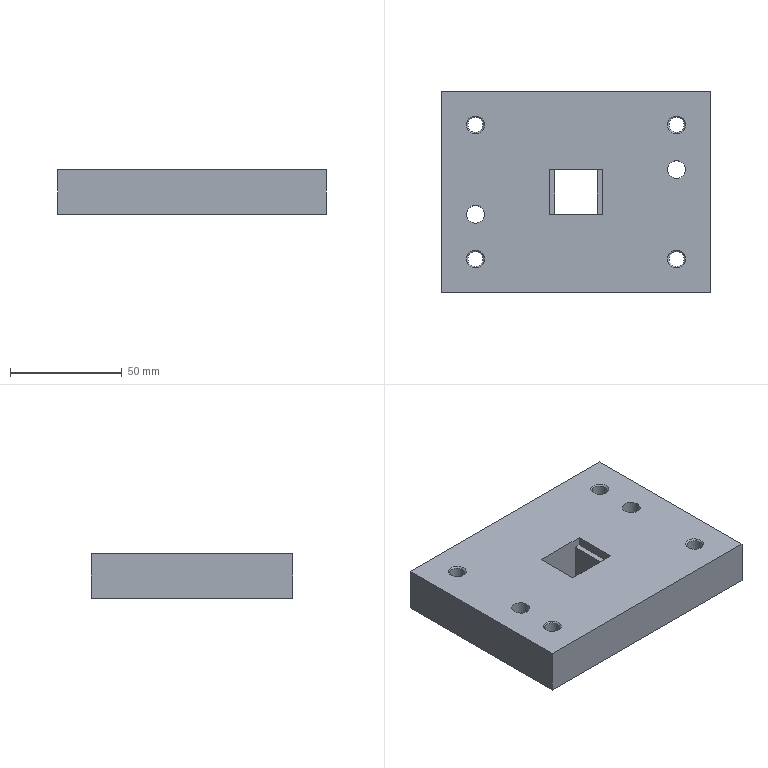Part | NX | features SIMPLE HOLE 4, SYMBOLIC_THREAD 4, EXTRUDE 2, DATUM_CSYS 1, HOLE PACKAGE 1 | 1 solid | 28 faces | box 120 x 90 x 20 mm | volume 203051 mm3 | plane 14 | cone 8 | cylinder 6 | commonest cylinder face diameters 6.8 x4 8 x2
STEP:
#1=CARTESIAN_POINT('',(-41.,-30.,0.));
#2=VERTEX_POINT('',#1);
#3=CARTESIAN_POINT('',(-45.,-30.,0.));
#4=DIRECTION('',(0.,0.,1.));
#5=DIRECTION('',(1.,0.,0.));
#6=AXIS2_PLACEMENT_3D('',#3,#4,#5);
#7=CIRCLE('',#6,4.);
#8=EDGE_CURVE('',#2,#2,#7,.F.);
#9=ORIENTED_EDGE('',*,*,#8,.T.);
#10=EDGE_LOOP('',(#9));
#11=FACE_BOUND('',#10,.T.);
#12=CARTESIAN_POINT('',(-41.,30.,0.));
#13=VERTEX_POINT('',#12);
#14=CARTESIAN_POINT('',(-45.,30.,0.));
#15=DIRECTION('',(0.,0.,1.));
#16=DIRECTION('',(1.,0.,0.));
#17=AXIS2_PLACEMENT_3D('',#14,#15,#16);
#18=CIRCLE('',#17,4.);
#19=EDGE_CURVE('',#13,#13,#18,.F.);
#20=ORIENTED_EDGE('',*,*,#19,.T.);
#21=EDGE_LOOP('',(#20));
#22=FACE_BOUND('',#21,.T.);
#23=CARTESIAN_POINT('',(49.,-30.,0.));
#24=VERTEX_POINT('',#23);
#25=CARTESIAN_POINT('',(45.,-30.,0.));
#26=DIRECTION('',(0.,0.,1.));
#27=DIRECTION('',(1.,0.,0.));
#28=AXIS2_PLACEMENT_3D('',#25,#26,#27);
#29=CIRCLE('',#28,4.);
#30=EDGE_CURVE('',#24,#24,#29,.F.);
#31=ORIENTED_EDGE('',*,*,#30,.T.);
#32=EDGE_LOOP('',(#31));
#33=FACE_BOUND('',#32,.T.);
#34=CARTESIAN_POINT('',(49.,30.,0.));
#35=VERTEX_POINT('',#34);
#36=CARTESIAN_POINT('',(45.,30.,0.));
#37=DIRECTION('',(0.,0.,1.));
#38=DIRECTION('',(1.,0.,0.));
#39=AXIS2_PLACEMENT_3D('',#36,#37,#38);
#40=CIRCLE('',#39,4.);
#41=EDGE_CURVE('',#35,#35,#40,.F.);
#42=ORIENTED_EDGE('',*,*,#41,.T.);
#43=EDGE_LOOP('',(#42));
#44=FACE_BOUND('',#43,.T.);
#45=CARTESIAN_POINT('',(60.,45.,0.));
#46=VERTEX_POINT('',#45);
#47=CARTESIAN_POINT('',(-60.,45.,0.));
#48=VERTEX_POINT('',#47);
#49=CARTESIAN_POINT('',(60.,45.,0.));
#50=DIRECTION('',(-1.,0.,0.));
#51=VECTOR('',#50,1000.);
#52=LINE('',#49,#51);
#53=EDGE_CURVE('',#46,#48,#52,.T.);
#54=ORIENTED_EDGE('',*,*,#53,.T.);
#55=CARTESIAN_POINT('',(-60.,-45.,0.));
#56=VERTEX_POINT('',#55);
#57=CARTESIAN_POINT('',(-60.,45.,0.));
#58=DIRECTION('',(0.,-1.,0.));
#59=VECTOR('',#58,1000.);
#60=LINE('',#57,#59);
#61=EDGE_CURVE('',#48,#56,#60,.T.);
#62=ORIENTED_EDGE('',*,*,#61,.T.);
#63=CARTESIAN_POINT('',(60.,-45.,0.));
#64=VERTEX_POINT('',#63);
#65=CARTESIAN_POINT('',(-60.,-45.,0.));
#66=DIRECTION('',(1.,0.,0.));
#67=VECTOR('',#66,1000.);
#68=LINE('',#65,#67);
#69=EDGE_CURVE('',#56,#64,#68,.T.);
#70=ORIENTED_EDGE('',*,*,#69,.T.);
#71=CARTESIAN_POINT('',(60.,-45.,0.));
#72=DIRECTION('',(0.,1.,0.));
#73=VECTOR('',#72,1000.);
#74=LINE('',#71,#73);
#75=EDGE_CURVE('',#64,#46,#74,.T.);
#76=ORIENTED_EDGE('',*,*,#75,.T.);
#77=EDGE_LOOP('',(#54,#62,#70,#76));
#78=FACE_BOUND('',#77,.T.);
#79=CARTESIAN_POINT('',(49.,10.,0.));
#80=VERTEX_POINT('',#79);
#81=CARTESIAN_POINT('',(45.,10.,0.));
#82=DIRECTION('',(0.,0.,1.));
#83=DIRECTION('',(1.,0.,0.));
#84=AXIS2_PLACEMENT_3D('',#81,#82,#83);
#85=CIRCLE('',#84,4.);
#86=EDGE_CURVE('',#80,#80,#85,.T.);
#87=ORIENTED_EDGE('',*,*,#86,.F.);
#88=EDGE_LOOP('',(#87));
#89=FACE_BOUND('',#88,.T.);
#90=CARTESIAN_POINT('',(-41.,-10.,0.));
#91=VERTEX_POINT('',#90);
#92=CARTESIAN_POINT('',(-45.,-10.,0.));
#93=DIRECTION('',(0.,0.,1.));
#94=DIRECTION('',(1.,0.,0.));
#95=AXIS2_PLACEMENT_3D('',#92,#93,#94);
#96=CIRCLE('',#95,4.);
#97=EDGE_CURVE('',#91,#91,#96,.T.);
#98=ORIENTED_EDGE('',*,*,#97,.F.);
#99=EDGE_LOOP('',(#98));
#100=FACE_BOUND('',#99,.T.);
#101=CARTESIAN_POINT('',(12.,-10.,0.));
#102=VERTEX_POINT('',#101);
#103=CARTESIAN_POINT('',(-12.,-10.,0.));
#104=VERTEX_POINT('',#103);
#105=CARTESIAN_POINT('',(9.5,-10.,0.));
#106=DIRECTION('',(-1.,0.,0.));
#107=VECTOR('',#106,1000.);
#108=LINE('',#105,#107);
#109=EDGE_CURVE('',#102,#104,#108,.T.);
#110=ORIENTED_EDGE('',*,*,#109,.T.);
#111=CARTESIAN_POINT('',(-12.,10.,0.));
#112=VERTEX_POINT('',#111);
#113=CARTESIAN_POINT('',(-12.,-10.,0.));
#114=DIRECTION('',(0.,1.,0.));
#115=VECTOR('',#114,1000.);
#116=LINE('',#113,#115);
#117=EDGE_CURVE('',#104,#112,#116,.T.);
#118=ORIENTED_EDGE('',*,*,#117,.T.);
#119=CARTESIAN_POINT('',(12.,10.,0.));
#120=VERTEX_POINT('',#119);
#121=CARTESIAN_POINT('',(-9.5,10.,0.));
#122=DIRECTION('',(1.,0.,0.));
#123=VECTOR('',#122,1000.);
#124=LINE('',#121,#123);
#125=EDGE_CURVE('',#112,#120,#124,.T.);
#126=ORIENTED_EDGE('',*,*,#125,.T.);
#127=CARTESIAN_POINT('',(12.,10.,0.));
#128=DIRECTION('',(0.,-1.,0.));
#129=VECTOR('',#128,1000.);
#130=LINE('',#127,#129);
#131=EDGE_CURVE('',#120,#102,#130,.T.);
#132=ORIENTED_EDGE('',*,*,#131,.T.);
#133=EDGE_LOOP('',(#110,#118,#126,#132));
#134=FACE_BOUND('',#133,.T.);
#135=CARTESIAN_POINT('',(45.,10.,0.));
#136=DIRECTION('',(0.,0.,1.));
#137=DIRECTION('',(1.,0.,0.));
#138=AXIS2_PLACEMENT_3D('',#135,#136,#137);
#139=PLANE('',#138);
#140=ADVANCED_FACE('',(#11,#22,#33,#44,#78,#89,#100,#134),#139,.T.);
#141=CARTESIAN_POINT('',(-9.5,-10.,-4.));
#142=VERTEX_POINT('',#141);
#143=CARTESIAN_POINT('',(-9.5,10.,-4.));
#144=VERTEX_POINT('',#143);
#145=CARTESIAN_POINT('',(-9.5,-10.,-4.));
#146=DIRECTION('',(0.,1.,0.));
#147=VECTOR('',#146,1000.);
#148=LINE('',#145,#147);
#149=EDGE_CURVE('',#142,#144,#148,.T.);
#150=ORIENTED_EDGE('',*,*,#149,.F.);
#151=CARTESIAN_POINT('',(-9.5,-10.,-20.));
#152=VERTEX_POINT('',#151);
#153=CARTESIAN_POINT('',(-9.5,-10.,-20.));
#154=DIRECTION('',(0.,0.,1.));
#155=VECTOR('',#154,1000.);
#156=LINE('',#153,#155);
#157=EDGE_CURVE('',#152,#142,#156,.T.);
#158=ORIENTED_EDGE('',*,*,#157,.F.);
#159=CARTESIAN_POINT('',(-9.5,10.,-20.));
#160=VERTEX_POINT('',#159);
#161=CARTESIAN_POINT('',(-9.5,-10.,-20.));
#162=DIRECTION('',(0.,1.,0.));
#163=VECTOR('',#162,1000.);
#164=LINE('',#161,#163);
#165=EDGE_CURVE('',#152,#160,#164,.T.);
#166=ORIENTED_EDGE('',*,*,#165,.T.);
#167=CARTESIAN_POINT('',(-9.5,10.,-20.));
#168=DIRECTION('',(0.,0.,1.));
#169=VECTOR('',#168,1000.);
#170=LINE('',#167,#169);
#171=EDGE_CURVE('',#160,#144,#170,.T.);
#172=ORIENTED_EDGE('',*,*,#171,.T.);
#173=EDGE_LOOP('',(#150,#158,#166,#172));
#174=FACE_BOUND('',#173,.T.);
#175=CARTESIAN_POINT('',(-9.5,-10.,-20.));
#176=DIRECTION('',(1.,0.,0.));
#177=DIRECTION('',(0.,0.,-1.));
#178=AXIS2_PLACEMENT_3D('',#175,#176,#177);
#179=PLANE('',#178);
#180=ADVANCED_FACE('',(#174),#179,.T.);
#181=CARTESIAN_POINT('',(9.5,10.,-20.));
#182=VERTEX_POINT('',#181);
#183=CARTESIAN_POINT('',(9.5,10.,-4.));
#184=VERTEX_POINT('',#183);
#185=CARTESIAN_POINT('',(9.5,10.,-20.));
#186=DIRECTION('',(0.,0.,1.));
#187=VECTOR('',#186,1000.);
#188=LINE('',#185,#187);
#189=EDGE_CURVE('',#182,#184,#188,.T.);
#190=ORIENTED_EDGE('',*,*,#189,.T.);
#191=CARTESIAN_POINT('',(12.,10.,-4.));
#192=VERTEX_POINT('',#191);
#193=CARTESIAN_POINT('',(-12.,10.,-4.));
#194=DIRECTION('',(1.,0.,0.));
#195=VECTOR('',#194,1000.);
#196=LINE('',#193,#195);
#197=EDGE_CURVE('',#184,#192,#196,.T.);
#198=ORIENTED_EDGE('',*,*,#197,.T.);
#199=CARTESIAN_POINT('',(12.,10.,-4.));
#200=DIRECTION('',(0.,0.,1.));
#201=VECTOR('',#200,1000.);
#202=LINE('',#199,#201);
#203=EDGE_CURVE('',#192,#120,#202,.T.);
#204=ORIENTED_EDGE('',*,*,#203,.T.);
#205=ORIENTED_EDGE('',*,*,#125,.F.);
#206=CARTESIAN_POINT('',(-12.,10.,-4.));
#207=VERTEX_POINT('',#206);
#208=CARTESIAN_POINT('',(-12.,10.,-4.));
#209=DIRECTION('',(0.,0.,1.));
#210=VECTOR('',#209,1000.);
#211=LINE('',#208,#210);
#212=EDGE_CURVE('',#207,#112,#211,.T.);
#213=ORIENTED_EDGE('',*,*,#212,.F.);
#214=CARTESIAN_POINT('',(-12.,10.,-4.));
#215=DIRECTION('',(1.,0.,0.));
#216=VECTOR('',#215,1000.);
#217=LINE('',#214,#216);
#218=EDGE_CURVE('',#207,#144,#217,.T.);
#219=ORIENTED_EDGE('',*,*,#218,.T.);
#220=ORIENTED_EDGE('',*,*,#171,.F.);
#221=CARTESIAN_POINT('',(-9.5,10.,-20.));
#222=DIRECTION('',(1.,0.,0.));
#223=VECTOR('',#222,1000.);
#224=LINE('',#221,#223);
#225=EDGE_CURVE('',#160,#182,#224,.T.);
#226=ORIENTED_EDGE('',*,*,#225,.T.);
#227=EDGE_LOOP('',(#190,#198,#204,#205,#213,#219,#220,#226));
#228=FACE_BOUND('',#227,.T.);
#229=CARTESIAN_POINT('',(-9.5,10.,-20.));
#230=DIRECTION('',(0.,-1.,0.));
#231=DIRECTION('',(0.,0.,-1.));
#232=AXIS2_PLACEMENT_3D('',#229,#230,#231);
#233=PLANE('',#232);
#234=ADVANCED_FACE('',(#228),#233,.T.);
#235=CARTESIAN_POINT('',(9.5,-10.,-4.));
#236=VERTEX_POINT('',#235);
#237=CARTESIAN_POINT('',(9.5,10.,-4.));
#238=DIRECTION('',(0.,-1.,0.));
#239=VECTOR('',#238,1000.);
#240=LINE('',#237,#239);
#241=EDGE_CURVE('',#184,#236,#240,.T.);
#242=ORIENTED_EDGE('',*,*,#241,.F.);
#243=ORIENTED_EDGE('',*,*,#189,.F.);
#244=CARTESIAN_POINT('',(9.5,-10.,-20.));
#245=VERTEX_POINT('',#244);
#246=CARTESIAN_POINT('',(9.5,10.,-20.));
#247=DIRECTION('',(0.,-1.,0.));
#248=VECTOR('',#247,1000.);
#249=LINE('',#246,#248);
#250=EDGE_CURVE('',#182,#245,#249,.T.);
#251=ORIENTED_EDGE('',*,*,#250,.T.);
#252=CARTESIAN_POINT('',(9.5,-10.,-20.));
#253=DIRECTION('',(0.,0.,1.));
#254=VECTOR('',#253,1000.);
#255=LINE('',#252,#254);
#256=EDGE_CURVE('',#245,#236,#255,.T.);
#257=ORIENTED_EDGE('',*,*,#256,.T.);
#258=EDGE_LOOP('',(#242,#243,#251,#257));
#259=FACE_BOUND('',#258,.T.);
#260=CARTESIAN_POINT('',(9.5,10.,-20.));
#261=DIRECTION('',(-1.,0.,0.));
#262=DIRECTION('',(0.,0.,1.));
#263=AXIS2_PLACEMENT_3D('',#260,#261,#262);
#264=PLANE('',#263);
#265=ADVANCED_FACE('',(#259),#264,.T.);
#266=ORIENTED_EDGE('',*,*,#53,.F.);
#267=CARTESIAN_POINT('',(60.,45.,-20.));
#268=VERTEX_POINT('',#267);
#269=CARTESIAN_POINT('',(60.,45.,-20.));
#270=DIRECTION('',(0.,0.,1.));
#271=VECTOR('',#270,1000.);
#272=LINE('',#269,#271);
#273=EDGE_CURVE('',#268,#46,#272,.T.);
#274=ORIENTED_EDGE('',*,*,#273,.F.);
#275=CARTESIAN_POINT('',(-60.,45.,-20.));
#276=VERTEX_POINT('',#275);
#277=CARTESIAN_POINT('',(60.,45.,-20.));
#278=DIRECTION('',(-1.,0.,0.));
#279=VECTOR('',#278,1000.);
#280=LINE('',#277,#279);
#281=EDGE_CURVE('',#268,#276,#280,.T.);
#282=ORIENTED_EDGE('',*,*,#281,.T.);
#283=CARTESIAN_POINT('',(-60.,45.,-20.));
#284=DIRECTION('',(0.,0.,1.));
#285=VECTOR('',#284,1000.);
#286=LINE('',#283,#285);
#287=EDGE_CURVE('',#276,#48,#286,.T.);
#288=ORIENTED_EDGE('',*,*,#287,.T.);
#289=EDGE_LOOP('',(#266,#274,#282,#288));
#290=FACE_BOUND('',#289,.T.);
#291=CARTESIAN_POINT('',(60.,45.,-20.));
#292=DIRECTION('',(0.,1.,0.));
#293=DIRECTION('',(0.,0.,1.));
#294=AXIS2_PLACEMENT_3D('',#291,#292,#293);
#295=PLANE('',#294);
#296=ADVANCED_FACE('',(#290),#295,.T.);
#297=ORIENTED_EDGE('',*,*,#61,.F.);
#298=ORIENTED_EDGE('',*,*,#287,.F.);
#299=CARTESIAN_POINT('',(-60.,-45.,-20.));
#300=VERTEX_POINT('',#299);
#301=CARTESIAN_POINT('',(-60.,45.,-20.));
#302=DIRECTION('',(0.,-1.,0.));
#303=VECTOR('',#302,1000.);
#304=LINE('',#301,#303);
#305=EDGE_CURVE('',#276,#300,#304,.T.);
#306=ORIENTED_EDGE('',*,*,#305,.T.);
#307=CARTESIAN_POINT('',(-60.,-45.,-20.));
#308=DIRECTION('',(0.,0.,1.));
#309=VECTOR('',#308,1000.);
#310=LINE('',#307,#309);
#311=EDGE_CURVE('',#300,#56,#310,.T.);
#312=ORIENTED_EDGE('',*,*,#311,.T.);
#313=EDGE_LOOP('',(#297,#298,#306,#312));
#314=FACE_BOUND('',#313,.T.);
#315=CARTESIAN_POINT('',(-60.,45.,-20.));
#316=DIRECTION('',(-1.,0.,0.));
#317=DIRECTION('',(0.,0.,1.));
#318=AXIS2_PLACEMENT_3D('',#315,#316,#317);
#319=PLANE('',#318);
#320=ADVANCED_FACE('',(#314),#319,.T.);
#321=ORIENTED_EDGE('',*,*,#69,.F.);
#322=ORIENTED_EDGE('',*,*,#311,.F.);
#323=CARTESIAN_POINT('',(60.,-45.,-20.));
#324=VERTEX_POINT('',#323);
#325=CARTESIAN_POINT('',(-60.,-45.,-20.));
#326=DIRECTION('',(1.,0.,0.));
#327=VECTOR('',#326,1000.);
#328=LINE('',#325,#327);
#329=EDGE_CURVE('',#300,#324,#328,.T.);
#330=ORIENTED_EDGE('',*,*,#329,.T.);
#331=CARTESIAN_POINT('',(60.,-45.,-20.));
#332=DIRECTION('',(0.,0.,1.));
#333=VECTOR('',#332,1000.);
#334=LINE('',#331,#333);
#335=EDGE_CURVE('',#324,#64,#334,.T.);
#336=ORIENTED_EDGE('',*,*,#335,.T.);
#337=EDGE_LOOP('',(#321,#322,#330,#336));
#338=FACE_BOUND('',#337,.T.);
#339=CARTESIAN_POINT('',(-60.,-45.,-20.));
#340=DIRECTION('',(0.,-1.,0.));
#341=DIRECTION('',(0.,0.,-1.));
#342=AXIS2_PLACEMENT_3D('',#339,#340,#341);
#343=PLANE('',#342);
#344=ADVANCED_FACE('',(#338),#343,.T.);
#345=CARTESIAN_POINT('',(-41.,-10.,-20.));
#346=VERTEX_POINT('',#345);
#347=CARTESIAN_POINT('',(-45.,-10.,-20.));
#348=DIRECTION('',(0.,0.,1.));
#349=DIRECTION('',(1.,0.,0.));
#350=AXIS2_PLACEMENT_3D('',#347,#348,#349);
#351=CIRCLE('',#350,4.);
#352=EDGE_CURVE('',#346,#346,#351,.T.);
#353=ORIENTED_EDGE('',*,*,#352,.F.);
#354=EDGE_LOOP('',(#353));
#355=FACE_BOUND('',#354,.T.);
#356=ORIENTED_EDGE('',*,*,#97,.T.);
#357=EDGE_LOOP('',(#356));
#358=FACE_BOUND('',#357,.T.);
#359=CARTESIAN_POINT('',(-45.,-10.,-20.));
#360=DIRECTION('',(0.,0.,1.));
#361=DIRECTION('',(1.,0.,0.));
#362=AXIS2_PLACEMENT_3D('',#359,#360,#361);
#363=CYLINDRICAL_SURFACE('',#362,4.);
#364=ADVANCED_FACE('',(#355,#358),#363,.F.);
#365=CARTESIAN_POINT('',(49.,10.,-20.));
#366=VERTEX_POINT('',#365);
#367=CARTESIAN_POINT('',(45.,10.,-20.));
#368=DIRECTION('',(0.,0.,1.));
#369=DIRECTION('',(1.,0.,0.));
#370=AXIS2_PLACEMENT_3D('',#367,#368,#369);
#371=CIRCLE('',#370,4.);
#372=EDGE_CURVE('',#366,#366,#371,.T.);
#373=ORIENTED_EDGE('',*,*,#372,.F.);
#374=EDGE_LOOP('',(#373));
#375=FACE_BOUND('',#374,.T.);
#376=ORIENTED_EDGE('',*,*,#86,.T.);
#377=EDGE_LOOP('',(#376));
#378=FACE_BOUND('',#377,.T.);
#379=CARTESIAN_POINT('',(45.,10.,-20.));
#380=DIRECTION('',(0.,0.,1.));
#381=DIRECTION('',(1.,0.,0.));
#382=AXIS2_PLACEMENT_3D('',#379,#380,#381);
#383=CYLINDRICAL_SURFACE('',#382,4.);
#384=ADVANCED_FACE('',(#375,#378),#383,.F.);
#385=ORIENTED_EDGE('',*,*,#75,.F.);
#386=ORIENTED_EDGE('',*,*,#335,.F.);
#387=CARTESIAN_POINT('',(60.,-45.,-20.));
#388=DIRECTION('',(0.,1.,0.));
#389=VECTOR('',#388,1000.);
#390=LINE('',#387,#389);
#391=EDGE_CURVE('',#324,#268,#390,.T.);
#392=ORIENTED_EDGE('',*,*,#391,.T.);
#393=ORIENTED_EDGE('',*,*,#273,.T.);
#394=EDGE_LOOP('',(#385,#386,#392,#393));
#395=FACE_BOUND('',#394,.T.);
#396=CARTESIAN_POINT('',(60.,-45.,-20.));
#397=DIRECTION('',(1.,0.,0.));
#398=DIRECTION('',(0.,0.,-1.));
#399=AXIS2_PLACEMENT_3D('',#396,#397,#398);
#400=PLANE('',#399);
#401=ADVANCED_FACE('',(#395),#400,.T.);
#402=ORIENTED_EDGE('',*,*,#157,.T.);
#403=CARTESIAN_POINT('',(-12.,-10.,-4.));
#404=VERTEX_POINT('',#403);
#405=CARTESIAN_POINT('',(-9.5,-10.,-4.));
#406=DIRECTION('',(-1.,0.,0.));
#407=VECTOR('',#406,1000.);
#408=LINE('',#405,#407);
#409=EDGE_CURVE('',#142,#404,#408,.T.);
#410=ORIENTED_EDGE('',*,*,#409,.T.);
#411=CARTESIAN_POINT('',(-12.,-10.,-4.));
#412=DIRECTION('',(0.,0.,1.));
#413=VECTOR('',#412,1000.);
#414=LINE('',#411,#413);
#415=EDGE_CURVE('',#404,#104,#414,.T.);
#416=ORIENTED_EDGE('',*,*,#415,.T.);
#417=ORIENTED_EDGE('',*,*,#109,.F.);
#418=CARTESIAN_POINT('',(12.,-10.,-4.));
#419=VERTEX_POINT('',#418);
#420=CARTESIAN_POINT('',(12.,-10.,-4.));
#421=DIRECTION('',(0.,0.,1.));
#422=VECTOR('',#421,1000.);
#423=LINE('',#420,#422);
#424=EDGE_CURVE('',#419,#102,#423,.T.);
#425=ORIENTED_EDGE('',*,*,#424,.F.);
#426=CARTESIAN_POINT('',(-9.5,-10.,-4.));
#427=DIRECTION('',(-1.,0.,0.));
#428=VECTOR('',#427,1000.);
#429=LINE('',#426,#428);
#430=EDGE_CURVE('',#419,#236,#429,.T.);
#431=ORIENTED_EDGE('',*,*,#430,.T.);
#432=ORIENTED_EDGE('',*,*,#256,.F.);
#433=CARTESIAN_POINT('',(9.5,-10.,-20.));
#434=DIRECTION('',(-1.,0.,0.));
#435=VECTOR('',#434,1000.);
#436=LINE('',#433,#435);
#437=EDGE_CURVE('',#245,#152,#436,.T.);
#438=ORIENTED_EDGE('',*,*,#437,.T.);
#439=EDGE_LOOP('',(#402,#410,#416,#417,#425,#431,#432,#438));
#440=FACE_BOUND('',#439,.T.);
#441=CARTESIAN_POINT('',(9.5,-10.,-20.));
#442=DIRECTION('',(0.,1.,0.));
#443=DIRECTION('',(-1.,0.,0.));
#444=AXIS2_PLACEMENT_3D('',#441,#442,#443);
#445=PLANE('',#444);
#446=ADVANCED_FACE('',(#440),#445,.T.);
#447=CARTESIAN_POINT('',(-41.,-30.,-20.));
#448=VERTEX_POINT('',#447);
#449=CARTESIAN_POINT('',(-45.,-30.,-20.));
#450=DIRECTION('',(0.,0.,1.));
#451=DIRECTION('',(1.,0.,0.));
#452=AXIS2_PLACEMENT_3D('',#449,#450,#451);
#453=CIRCLE('',#452,4.);
#454=EDGE_CURVE('',#448,#448,#453,.T.);
#455=ORIENTED_EDGE('',*,*,#454,.T.);
#456=EDGE_LOOP('',(#455));
#457=FACE_BOUND('',#456,.T.);
#458=CARTESIAN_POINT('',(-41.,30.,-20.));
#459=VERTEX_POINT('',#458);
#460=CARTESIAN_POINT('',(-45.,30.,-20.));
#461=DIRECTION('',(0.,0.,1.));
#462=DIRECTION('',(1.,0.,0.));
#463=AXIS2_PLACEMENT_3D('',#460,#461,#462);
#464=CIRCLE('',#463,4.);
#465=EDGE_CURVE('',#459,#459,#464,.T.);
#466=ORIENTED_EDGE('',*,*,#465,.T.);
#467=EDGE_LOOP('',(#466));
#468=FACE_BOUND('',#467,.T.);
#469=CARTESIAN_POINT('',(49.,-30.,-20.));
#470=VERTEX_POINT('',#469);
#471=CARTESIAN_POINT('',(45.,-30.,-20.));
#472=DIRECTION('',(0.,0.,1.));
#473=DIRECTION('',(1.,0.,0.));
#474=AXIS2_PLACEMENT_3D('',#471,#472,#473);
#475=CIRCLE('',#474,4.);
#476=EDGE_CURVE('',#470,#470,#475,.T.);
#477=ORIENTED_EDGE('',*,*,#476,.T.);
#478=EDGE_LOOP('',(#477));
#479=FACE_BOUND('',#478,.T.);
#480=CARTESIAN_POINT('',(49.,30.,-20.));
#481=VERTEX_POINT('',#480);
#482=CARTESIAN_POINT('',(45.,30.,-20.));
#483=DIRECTION('',(0.,0.,1.));
#484=DIRECTION('',(1.,0.,0.));
#485=AXIS2_PLACEMENT_3D('',#482,#483,#484);
#486=CIRCLE('',#485,4.);
#487=EDGE_CURVE('',#481,#481,#486,.T.);
#488=ORIENTED_EDGE('',*,*,#487,.T.);
#489=EDGE_LOOP('',(#488));
#490=FACE_BOUND('',#489,.T.);
#491=ORIENTED_EDGE('',*,*,#281,.F.);
#492=ORIENTED_EDGE('',*,*,#391,.F.);
#493=ORIENTED_EDGE('',*,*,#329,.F.);
#494=ORIENTED_EDGE('',*,*,#305,.F.);
#495=EDGE_LOOP('',(#491,#492,#493,#494));
#496=FACE_BOUND('',#495,.T.);
#497=ORIENTED_EDGE('',*,*,#372,.T.);
#498=EDGE_LOOP('',(#497));
#499=FACE_BOUND('',#498,.T.);
#500=ORIENTED_EDGE('',*,*,#352,.T.);
#501=EDGE_LOOP('',(#500));
#502=FACE_BOUND('',#501,.T.);
#503=ORIENTED_EDGE('',*,*,#165,.F.);
#504=ORIENTED_EDGE('',*,*,#437,.F.);
#505=ORIENTED_EDGE('',*,*,#250,.F.);
#506=ORIENTED_EDGE('',*,*,#225,.F.);
#507=EDGE_LOOP('',(#503,#504,#505,#506));
#508=FACE_BOUND('',#507,.T.);
#509=CARTESIAN_POINT('',(45.,10.,-20.));
#510=DIRECTION('',(0.,0.,1.));
#511=DIRECTION('',(1.,0.,0.));
#512=AXIS2_PLACEMENT_3D('',#509,#510,#511);
#513=PLANE('',#512);
#514=ADVANCED_FACE('',(#457,#468,#479,#490,#496,#499,#502,#508),#513,.F.);
#515=ORIENTED_EDGE('',*,*,#241,.T.);
#516=ORIENTED_EDGE('',*,*,#430,.F.);
#517=CARTESIAN_POINT('',(12.,10.,-4.));
#518=DIRECTION('',(0.,-1.,0.));
#519=VECTOR('',#518,1000.);
#520=LINE('',#517,#519);
#521=EDGE_CURVE('',#419,#192,#520,.F.);
#522=ORIENTED_EDGE('',*,*,#521,.T.);
#523=ORIENTED_EDGE('',*,*,#197,.F.);
#524=EDGE_LOOP('',(#515,#516,#522,#523));
#525=FACE_BOUND('',#524,.T.);
#526=CARTESIAN_POINT('',(0.,0.,-4.));
#527=DIRECTION('',(0.,0.,-1.));
#528=DIRECTION('',(-1.,0.,0.));
#529=AXIS2_PLACEMENT_3D('',#526,#527,#528);
#530=PLANE('',#529);
#531=ADVANCED_FACE('',(#525),#530,.F.);
#532=ORIENTED_EDGE('',*,*,#131,.F.);
#533=ORIENTED_EDGE('',*,*,#203,.F.);
#534=ORIENTED_EDGE('',*,*,#521,.F.);
#535=ORIENTED_EDGE('',*,*,#424,.T.);
#536=EDGE_LOOP('',(#532,#533,#534,#535));
#537=FACE_BOUND('',#536,.T.);
#538=CARTESIAN_POINT('',(12.,10.,-4.));
#539=DIRECTION('',(-1.,0.,0.));
#540=DIRECTION('',(0.,0.,1.));
#541=AXIS2_PLACEMENT_3D('',#538,#539,#540);
#542=PLANE('',#541);
#543=ADVANCED_FACE('',(#537),#542,.T.);
#544=ORIENTED_EDGE('',*,*,#149,.T.);
#545=ORIENTED_EDGE('',*,*,#218,.F.);
#546=CARTESIAN_POINT('',(-12.,-10.,-4.));
#547=DIRECTION('',(0.,1.,0.));
#548=VECTOR('',#547,1000.);
#549=LINE('',#546,#548);
#550=EDGE_CURVE('',#207,#404,#549,.F.);
#551=ORIENTED_EDGE('',*,*,#550,.T.);
#552=ORIENTED_EDGE('',*,*,#409,.F.);
#553=EDGE_LOOP('',(#544,#545,#551,#552));
#554=FACE_BOUND('',#553,.T.);
#555=CARTESIAN_POINT('',(0.,0.,-4.));
#556=DIRECTION('',(0.,0.,-1.));
#557=DIRECTION('',(-1.,0.,0.));
#558=AXIS2_PLACEMENT_3D('',#555,#556,#557);
#559=PLANE('',#558);
#560=ADVANCED_FACE('',(#554),#559,.F.);
#561=ORIENTED_EDGE('',*,*,#117,.F.);
#562=ORIENTED_EDGE('',*,*,#415,.F.);
#563=ORIENTED_EDGE('',*,*,#550,.F.);
#564=ORIENTED_EDGE('',*,*,#212,.T.);
#565=EDGE_LOOP('',(#561,#562,#563,#564));
#566=FACE_BOUND('',#565,.T.);
#567=CARTESIAN_POINT('',(-12.,-10.,-4.));
#568=DIRECTION('',(1.,0.,0.));
#569=DIRECTION('',(0.,0.,-1.));
#570=AXIS2_PLACEMENT_3D('',#567,#568,#569);
#571=PLANE('',#570);
#572=ADVANCED_FACE('',(#566),#571,.T.);
#573=CARTESIAN_POINT('',(48.4,30.,-19.4));
#574=VERTEX_POINT('',#573);
#575=CARTESIAN_POINT('',(45.,30.,-19.4));
#576=DIRECTION('',(0.,0.,1.));
#577=DIRECTION('',(1.,0.,0.));
#578=AXIS2_PLACEMENT_3D('',#575,#576,#577);
#579=CIRCLE('',#578,3.4);
#580=EDGE_CURVE('',#574,#574,#579,.F.);
#581=ORIENTED_EDGE('',*,*,#580,.T.);
#582=EDGE_LOOP('',(#581));
#583=FACE_BOUND('',#582,.T.);
#584=CARTESIAN_POINT('',(48.4,30.,-0.6));
#585=VERTEX_POINT('',#584);
#586=CARTESIAN_POINT('',(45.,30.,-0.6));
#587=DIRECTION('',(0.,0.,1.));
#588=DIRECTION('',(1.,0.,0.));
#589=AXIS2_PLACEMENT_3D('',#586,#587,#588);
#590=CIRCLE('',#589,3.4);
#591=EDGE_CURVE('',#585,#585,#590,.T.);
#592=ORIENTED_EDGE('',*,*,#591,.T.);
#593=EDGE_LOOP('',(#592));
#594=FACE_BOUND('',#593,.T.);
#595=CARTESIAN_POINT('',(45.,30.,0.));
#596=DIRECTION('',(0.,0.,-1.));
#597=DIRECTION('',(-1.,0.,0.));
#598=AXIS2_PLACEMENT_3D('',#595,#596,#597);
#599=CYLINDRICAL_SURFACE('',#598,3.4);
#600=ADVANCED_FACE('',(#583,#594),#599,.F.);
#601=ORIENTED_EDGE('',*,*,#591,.F.);
#602=EDGE_LOOP('',(#601));
#603=FACE_BOUND('',#602,.T.);
#604=ORIENTED_EDGE('',*,*,#41,.F.);
#605=EDGE_LOOP('',(#604));
#606=FACE_BOUND('',#605,.T.);
#607=CARTESIAN_POINT('',(45.,30.,0.));
#608=DIRECTION('',(0.,0.,1.));
#609=DIRECTION('',(1.,0.,0.));
#610=AXIS2_PLACEMENT_3D('',#607,#608,#609);
#611=CONICAL_SURFACE('',#610,4.,0.7854);
#612=ADVANCED_FACE('',(#603,#606),#611,.F.);
#613=ORIENTED_EDGE('',*,*,#580,.F.);
#614=EDGE_LOOP('',(#613));
#615=FACE_BOUND('',#614,.T.);
#616=ORIENTED_EDGE('',*,*,#487,.F.);
#617=EDGE_LOOP('',(#616));
#618=FACE_BOUND('',#617,.T.);
#619=CARTESIAN_POINT('',(45.,30.,-20.));
#620=DIRECTION('',(0.,0.,-1.));
#621=DIRECTION('',(-1.,0.,0.));
#622=AXIS2_PLACEMENT_3D('',#619,#620,#621);
#623=CONICAL_SURFACE('',#622,4.,0.7854);
#624=ADVANCED_FACE('',(#615,#618),#623,.F.);
#625=CARTESIAN_POINT('',(48.4,-30.,-19.4));
#626=VERTEX_POINT('',#625);
#627=CARTESIAN_POINT('',(45.,-30.,-19.4));
#628=DIRECTION('',(0.,0.,1.));
#629=DIRECTION('',(1.,0.,0.));
#630=AXIS2_PLACEMENT_3D('',#627,#628,#629);
#631=CIRCLE('',#630,3.4);
#632=EDGE_CURVE('',#626,#626,#631,.F.);
#633=ORIENTED_EDGE('',*,*,#632,.T.);
#634=EDGE_LOOP('',(#633));
#635=FACE_BOUND('',#634,.T.);
#636=CARTESIAN_POINT('',(48.4,-30.,-0.6));
#637=VERTEX_POINT('',#636);
#638=CARTESIAN_POINT('',(45.,-30.,-0.6));
#639=DIRECTION('',(0.,0.,1.));
#640=DIRECTION('',(1.,0.,0.));
#641=AXIS2_PLACEMENT_3D('',#638,#639,#640);
#642=CIRCLE('',#641,3.4);
#643=EDGE_CURVE('',#637,#637,#642,.T.);
#644=ORIENTED_EDGE('',*,*,#643,.T.);
#645=EDGE_LOOP('',(#644));
#646=FACE_BOUND('',#645,.T.);
#647=CARTESIAN_POINT('',(45.,-30.,0.));
#648=DIRECTION('',(0.,0.,-1.));
#649=DIRECTION('',(-1.,0.,0.));
#650=AXIS2_PLACEMENT_3D('',#647,#648,#649);
#651=CYLINDRICAL_SURFACE('',#650,3.4);
#652=ADVANCED_FACE('',(#635,#646),#651,.F.);
#653=ORIENTED_EDGE('',*,*,#643,.F.);
#654=EDGE_LOOP('',(#653));
#655=FACE_BOUND('',#654,.T.);
#656=ORIENTED_EDGE('',*,*,#30,.F.);
#657=EDGE_LOOP('',(#656));
#658=FACE_BOUND('',#657,.T.);
#659=CARTESIAN_POINT('',(45.,-30.,0.));
#660=DIRECTION('',(0.,0.,1.));
#661=DIRECTION('',(1.,0.,0.));
#662=AXIS2_PLACEMENT_3D('',#659,#660,#661);
#663=CONICAL_SURFACE('',#662,4.,0.7854);
#664=ADVANCED_FACE('',(#655,#658),#663,.F.);
#665=ORIENTED_EDGE('',*,*,#632,.F.);
#666=EDGE_LOOP('',(#665));
#667=FACE_BOUND('',#666,.T.);
#668=ORIENTED_EDGE('',*,*,#476,.F.);
#669=EDGE_LOOP('',(#668));
#670=FACE_BOUND('',#669,.T.);
#671=CARTESIAN_POINT('',(45.,-30.,-20.));
#672=DIRECTION('',(0.,0.,-1.));
#673=DIRECTION('',(-1.,0.,0.));
#674=AXIS2_PLACEMENT_3D('',#671,#672,#673);
#675=CONICAL_SURFACE('',#674,4.,0.7854);
#676=ADVANCED_FACE('',(#667,#670),#675,.F.);
#677=CARTESIAN_POINT('',(-41.6,30.,-19.4));
#678=VERTEX_POINT('',#677);
#679=CARTESIAN_POINT('',(-45.,30.,-19.4));
#680=DIRECTION('',(0.,0.,1.));
#681=DIRECTION('',(1.,0.,0.));
#682=AXIS2_PLACEMENT_3D('',#679,#680,#681);
#683=CIRCLE('',#682,3.4);
#684=EDGE_CURVE('',#678,#678,#683,.F.);
#685=ORIENTED_EDGE('',*,*,#684,.T.);
#686=EDGE_LOOP('',(#685));
#687=FACE_BOUND('',#686,.T.);
#688=CARTESIAN_POINT('',(-41.6,30.,-0.6));
#689=VERTEX_POINT('',#688);
#690=CARTESIAN_POINT('',(-45.,30.,-0.6));
#691=DIRECTION('',(0.,0.,1.));
#692=DIRECTION('',(1.,0.,0.));
#693=AXIS2_PLACEMENT_3D('',#690,#691,#692);
#694=CIRCLE('',#693,3.4);
#695=EDGE_CURVE('',#689,#689,#694,.T.);
#696=ORIENTED_EDGE('',*,*,#695,.T.);
#697=EDGE_LOOP('',(#696));
#698=FACE_BOUND('',#697,.T.);
#699=CARTESIAN_POINT('',(-45.,30.,0.));
#700=DIRECTION('',(0.,0.,-1.));
#701=DIRECTION('',(-1.,0.,0.));
#702=AXIS2_PLACEMENT_3D('',#699,#700,#701);
#703=CYLINDRICAL_SURFACE('',#702,3.4);
#704=ADVANCED_FACE('',(#687,#698),#703,.F.);
#705=ORIENTED_EDGE('',*,*,#695,.F.);
#706=EDGE_LOOP('',(#705));
#707=FACE_BOUND('',#706,.T.);
#708=ORIENTED_EDGE('',*,*,#19,.F.);
#709=EDGE_LOOP('',(#708));
#710=FACE_BOUND('',#709,.T.);
#711=CARTESIAN_POINT('',(-45.,30.,0.));
#712=DIRECTION('',(0.,0.,1.));
#713=DIRECTION('',(1.,0.,0.));
#714=AXIS2_PLACEMENT_3D('',#711,#712,#713);
#715=CONICAL_SURFACE('',#714,4.,0.7854);
#716=ADVANCED_FACE('',(#707,#710),#715,.F.);
#717=ORIENTED_EDGE('',*,*,#684,.F.);
#718=EDGE_LOOP('',(#717));
#719=FACE_BOUND('',#718,.T.);
#720=ORIENTED_EDGE('',*,*,#465,.F.);
#721=EDGE_LOOP('',(#720));
#722=FACE_BOUND('',#721,.T.);
#723=CARTESIAN_POINT('',(-45.,30.,-20.));
#724=DIRECTION('',(0.,0.,-1.));
#725=DIRECTION('',(-1.,0.,0.));
#726=AXIS2_PLACEMENT_3D('',#723,#724,#725);
#727=CONICAL_SURFACE('',#726,4.,0.7854);
#728=ADVANCED_FACE('',(#719,#722),#727,.F.);
#729=CARTESIAN_POINT('',(-41.6,-30.,-19.4));
#730=VERTEX_POINT('',#729);
#731=CARTESIAN_POINT('',(-45.,-30.,-19.4));
#732=DIRECTION('',(0.,0.,1.));
#733=DIRECTION('',(1.,0.,0.));
#734=AXIS2_PLACEMENT_3D('',#731,#732,#733);
#735=CIRCLE('',#734,3.4);
#736=EDGE_CURVE('',#730,#730,#735,.F.);
#737=ORIENTED_EDGE('',*,*,#736,.T.);
#738=EDGE_LOOP('',(#737));
#739=FACE_BOUND('',#738,.T.);
#740=CARTESIAN_POINT('',(-41.6,-30.,-0.6));
#741=VERTEX_POINT('',#740);
#742=CARTESIAN_POINT('',(-45.,-30.,-0.6));
#743=DIRECTION('',(0.,0.,1.));
#744=DIRECTION('',(1.,0.,0.));
#745=AXIS2_PLACEMENT_3D('',#742,#743,#744);
#746=CIRCLE('',#745,3.4);
#747=EDGE_CURVE('',#741,#741,#746,.T.);
#748=ORIENTED_EDGE('',*,*,#747,.T.);
#749=EDGE_LOOP('',(#748));
#750=FACE_BOUND('',#749,.T.);
#751=CARTESIAN_POINT('',(-45.,-30.,0.));
#752=DIRECTION('',(0.,0.,-1.));
#753=DIRECTION('',(-1.,0.,0.));
#754=AXIS2_PLACEMENT_3D('',#751,#752,#753);
#755=CYLINDRICAL_SURFACE('',#754,3.4);
#756=ADVANCED_FACE('',(#739,#750),#755,.F.);
#757=ORIENTED_EDGE('',*,*,#747,.F.);
#758=EDGE_LOOP('',(#757));
#759=FACE_BOUND('',#758,.T.);
#760=ORIENTED_EDGE('',*,*,#8,.F.);
#761=EDGE_LOOP('',(#760));
#762=FACE_BOUND('',#761,.T.);
#763=CARTESIAN_POINT('',(-45.,-30.,0.));
#764=DIRECTION('',(0.,0.,1.));
#765=DIRECTION('',(1.,0.,0.));
#766=AXIS2_PLACEMENT_3D('',#763,#764,#765);
#767=CONICAL_SURFACE('',#766,4.,0.7854);
#768=ADVANCED_FACE('',(#759,#762),#767,.F.);
#769=ORIENTED_EDGE('',*,*,#736,.F.);
#770=EDGE_LOOP('',(#769));
#771=FACE_BOUND('',#770,.T.);
#772=ORIENTED_EDGE('',*,*,#454,.F.);
#773=EDGE_LOOP('',(#772));
#774=FACE_BOUND('',#773,.T.);
#775=CARTESIAN_POINT('',(-45.,-30.,-20.));
#776=DIRECTION('',(0.,0.,-1.));
#777=DIRECTION('',(-1.,0.,0.));
#778=AXIS2_PLACEMENT_3D('',#775,#776,#777);
#779=CONICAL_SURFACE('',#778,4.,0.7854);
#780=ADVANCED_FACE('',(#771,#774),#779,.F.);
#781=CLOSED_SHELL('',(#140,#180,#234,#265,#296,#320,#344,#364,#384,#401,#446,#514,#531,#543,#560,#572,#600,#612,#624,#652,#664,#676,#704,#716,#728,#756,#768,#780));
#782=MANIFOLD_SOLID_BREP('',#781);
#783=(LENGTH_UNIT()NAMED_UNIT(*)SI_UNIT(.MILLI.,.METRE.));
#784=UNCERTAINTY_MEASURE_WITH_UNIT(LENGTH_MEASURE(0.00001),#783,'','');
#785=(NAMED_UNIT(*)PLANE_ANGLE_UNIT()SI_UNIT($,.RADIAN.));
#786=(NAMED_UNIT(*)SI_UNIT($,.STERADIAN.)SOLID_ANGLE_UNIT());
#787=(GEOMETRIC_REPRESENTATION_CONTEXT(3)GLOBAL_UNCERTAINTY_ASSIGNED_CONTEXT((#784))GLOBAL_UNIT_ASSIGNED_CONTEXT((#783,#785,#786))REPRESENTATION_CONTEXT('',''));
#788=ADVANCED_BREP_SHAPE_REPRESENTATION('',(#782),#787);